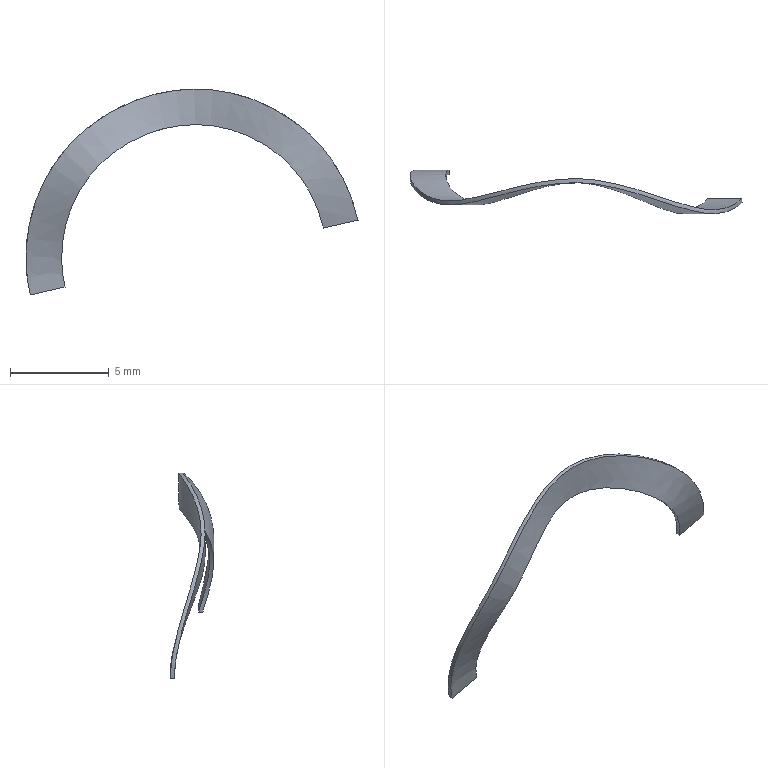Part | NX | features ODD_TURNS_COMBINE 2 | 1 solid | 6 faces | box 16.822 x 2.216 x 10.434 mm | volume 8.771 mm3 | spline 4 | plane 2
STEP:
#1=CARTESIAN_POINT('',(-6.562,-23.97,-1.498));
#2=VERTEX_POINT('',#1);
#3=CARTESIAN_POINT('',(-6.562,-24.173,-1.498));
#4=VERTEX_POINT('',#3);
#5=CARTESIAN_POINT('',(-6.562,-24.173,-1.498));
#6=CARTESIAN_POINT('',(-6.562,-24.105,-1.498));
#7=CARTESIAN_POINT('',(-6.562,-24.037,-1.498));
#8=CARTESIAN_POINT('',(-6.562,-23.97,-1.498));
#9=B_SPLINE_CURVE_WITH_KNOTS('',3,(#5,#6,#7,#8),.UNSPECIFIED.,.F.,.F.,(4,4),(0.000001219,0.0002044),.UNSPECIFIED.);
#10=EDGE_CURVE('',#2,#4,#9,.F.);
#11=ORIENTED_EDGE('',*,*,#10,.T.);
#12=CARTESIAN_POINT('',(-8.32,-24.173,-1.899));
#13=VERTEX_POINT('',#12);
#14=CARTESIAN_POINT('',(-8.32,-24.173,-1.899));
#15=CARTESIAN_POINT('',(-7.734,-24.173,-1.765));
#16=CARTESIAN_POINT('',(-7.148,-24.173,-1.631));
#17=CARTESIAN_POINT('',(-6.562,-24.173,-1.498));
#18=B_SPLINE_CURVE_WITH_KNOTS('',3,(#14,#15,#16,#17),.UNSPECIFIED.,.F.,.F.,(4,4),(0.,0.001803),.UNSPECIFIED.);
#19=EDGE_CURVE('',#4,#13,#18,.F.);
#20=ORIENTED_EDGE('',*,*,#19,.T.);
#21=CARTESIAN_POINT('',(-8.32,-23.97,-1.899));
#22=VERTEX_POINT('',#21);
#23=CARTESIAN_POINT('',(-8.32,-23.97,-1.899));
#24=CARTESIAN_POINT('',(-8.32,-24.037,-1.899));
#25=CARTESIAN_POINT('',(-8.32,-24.105,-1.899));
#26=CARTESIAN_POINT('',(-8.32,-24.173,-1.899));
#27=B_SPLINE_CURVE_WITH_KNOTS('',3,(#23,#24,#25,#26),.UNSPECIFIED.,.F.,.F.,(4,4),(0.,0.0002032),.UNSPECIFIED.);
#28=EDGE_CURVE('',#22,#13,#27,.T.);
#29=ORIENTED_EDGE('',*,*,#28,.F.);
#30=CARTESIAN_POINT('',(-6.562,-23.97,-1.498));
#31=CARTESIAN_POINT('',(-7.148,-23.97,-1.631));
#32=CARTESIAN_POINT('',(-7.734,-23.97,-1.765));
#33=CARTESIAN_POINT('',(-8.32,-23.97,-1.899));
#34=B_SPLINE_CURVE_WITH_KNOTS('',3,(#30,#31,#32,#33),.UNSPECIFIED.,.F.,.F.,(4,4),(0.,0.001803),.UNSPECIFIED.);
#35=EDGE_CURVE('',#22,#2,#34,.F.);
#36=ORIENTED_EDGE('',*,*,#35,.T.);
#37=EDGE_LOOP('',(#11,#20,#29,#36));
#38=FACE_BOUND('',#37,.T.);
#39=CARTESIAN_POINT('',(-8.32,-23.761,-1.899));
#40=DIRECTION('',(0.2225,0.,-0.9749));
#41=DIRECTION('',(-0.9749,0.,-0.2225));
#42=AXIS2_PLACEMENT_3D('',#39,#40,#41);
#43=PLANE('',#42);
#44=ADVANCED_FACE('',(#38),#43,.T.);
#45=CARTESIAN_POINT('',(8.284,-25.419,1.891));
#46=VERTEX_POINT('',#45);
#47=CARTESIAN_POINT('',(-3.703,-25.301,-7.689));
#48=CARTESIAN_POINT('',(-1.417,-25.248,-8.753));
#49=CARTESIAN_POINT('',(4.289,-27.759,-8.773));
#50=CARTESIAN_POINT('',(9.501,-23.516,-2.229));
#51=CARTESIAN_POINT('',(7.592,-27.322,6.131));
#52=CARTESIAN_POINT('',(0.06027,-23.071,9.76));
#53=CARTESIAN_POINT('',(-7.667,-26.878,6.037));
#54=CARTESIAN_POINT('',(-9.528,-22.627,-2.113));
#55=CARTESIAN_POINT('',(-4.18,-26.435,-8.819));
#56=CARTESIAN_POINT('',(4.18,-22.183,-8.819));
#57=CARTESIAN_POINT('',(9.527,-25.991,-2.113));
#58=CARTESIAN_POINT('',(7.668,-21.74,6.038));
#59=CARTESIAN_POINT('',(-0.06063,-25.547,9.759));
#60=CARTESIAN_POINT('',(-7.591,-21.298,6.133));
#61=CARTESIAN_POINT('',(-8.865,-23.825,0.5668));
#62=CARTESIAN_POINT('',(-8.32,-23.761,-1.899));
#63=B_SPLINE_CURVE_WITH_KNOTS('',3,(#47,#48,#49,#50,#51,#52,#53,#54,#55,#56,#57,#58,#59,#60,#61,#62),.UNSPECIFIED.,.F.,.F.,(4,1,1,1,1,1,1,1,1,1,1,1,1,4),(0.,0.07646,0.1539,0.2304,0.3078,0.3843,0.4618,0.5382,0.6157,0.6922,0.7696,0.8461,0.9235,1.),.UNSPECIFIED.);
#64=EDGE_CURVE('',#46,#22,#63,.T.);
#65=ORIENTED_EDGE('',*,*,#64,.T.);
#66=ORIENTED_EDGE('',*,*,#28,.T.);
#67=CARTESIAN_POINT('',(8.284,-25.622,1.891));
#68=VERTEX_POINT('',#67);
#69=CARTESIAN_POINT('',(-3.703,-25.504,-7.689));
#70=CARTESIAN_POINT('',(-1.417,-25.451,-8.753));
#71=CARTESIAN_POINT('',(4.289,-27.962,-8.773));
#72=CARTESIAN_POINT('',(9.501,-23.72,-2.229));
#73=CARTESIAN_POINT('',(7.592,-27.525,6.131));
#74=CARTESIAN_POINT('',(0.06027,-23.274,9.76));
#75=CARTESIAN_POINT('',(-7.667,-27.082,6.037));
#76=CARTESIAN_POINT('',(-9.528,-22.83,-2.113));
#77=CARTESIAN_POINT('',(-4.18,-26.638,-8.819));
#78=CARTESIAN_POINT('',(4.18,-22.387,-8.819));
#79=CARTESIAN_POINT('',(9.527,-26.194,-2.113));
#80=CARTESIAN_POINT('',(7.668,-21.943,6.038));
#81=CARTESIAN_POINT('',(-0.06063,-25.75,9.759));
#82=CARTESIAN_POINT('',(-7.591,-21.501,6.133));
#83=CARTESIAN_POINT('',(-8.865,-24.028,0.5668));
#84=CARTESIAN_POINT('',(-8.32,-23.964,-1.899));
#85=B_SPLINE_CURVE_WITH_KNOTS('',3,(#69,#70,#71,#72,#73,#74,#75,#76,#77,#78,#79,#80,#81,#82,#83,#84),.UNSPECIFIED.,.F.,.F.,(4,1,1,1,1,1,1,1,1,1,1,1,1,4),(0.,0.07646,0.1539,0.2304,0.3078,0.3843,0.4618,0.5382,0.6157,0.6922,0.7696,0.8461,0.9235,1.),.UNSPECIFIED.);
#86=EDGE_CURVE('',#68,#13,#85,.T.);
#87=ORIENTED_EDGE('',*,*,#86,.F.);
#88=CARTESIAN_POINT('',(8.284,-25.622,1.891));
#89=CARTESIAN_POINT('',(8.284,-25.554,1.891));
#90=CARTESIAN_POINT('',(8.284,-25.486,1.891));
#91=CARTESIAN_POINT('',(8.284,-25.419,1.891));
#92=B_SPLINE_CURVE_WITH_KNOTS('',3,(#88,#89,#90,#91),.UNSPECIFIED.,.F.,.F.,(4,4),(0.,0.0002032),.UNSPECIFIED.);
#93=EDGE_CURVE('',#68,#46,#92,.T.);
#94=ORIENTED_EDGE('',*,*,#93,.T.);
#95=EDGE_LOOP('',(#65,#66,#87,#94));
#96=FACE_BOUND('',#95,.T.);
#97=CARTESIAN_POINT('',(8.284,-25.622,1.891));
#98=CARTESIAN_POINT('',(7.999,-25.92,3.139));
#99=CARTESIAN_POINT('',(6.343,-26.82,6.733));
#100=CARTESIAN_POINT('',(0.06027,-23.274,9.76));
#101=CARTESIAN_POINT('',(-7.667,-27.082,6.037));
#102=CARTESIAN_POINT('',(-8.91,-24.241,0.5921));
#103=CARTESIAN_POINT('',(-8.32,-24.173,-1.899));
#104=CARTESIAN_POINT('',(8.284,-25.605,1.891));
#105=CARTESIAN_POINT('',(7.999,-25.903,3.139));
#106=CARTESIAN_POINT('',(6.343,-26.803,6.733));
#107=CARTESIAN_POINT('',(0.06027,-23.257,9.76));
#108=CARTESIAN_POINT('',(-7.667,-27.065,6.037));
#109=CARTESIAN_POINT('',(-8.91,-24.224,0.5921));
#110=CARTESIAN_POINT('',(-8.32,-24.156,-1.899));
#111=CARTESIAN_POINT('',(8.284,-25.571,1.891));
#112=CARTESIAN_POINT('',(7.999,-25.869,3.139));
#113=CARTESIAN_POINT('',(6.343,-26.769,6.733));
#114=CARTESIAN_POINT('',(0.06027,-23.223,9.76));
#115=CARTESIAN_POINT('',(-7.667,-27.031,6.037));
#116=CARTESIAN_POINT('',(-8.91,-24.19,0.5921));
#117=CARTESIAN_POINT('',(-8.32,-24.122,-1.899));
#118=CARTESIAN_POINT('',(8.284,-25.52,1.891));
#119=CARTESIAN_POINT('',(7.999,-25.818,3.139));
#120=CARTESIAN_POINT('',(6.343,-26.718,6.733));
#121=CARTESIAN_POINT('',(0.06027,-23.173,9.76));
#122=CARTESIAN_POINT('',(-7.667,-26.98,6.037));
#123=CARTESIAN_POINT('',(-8.91,-24.14,0.5921));
#124=CARTESIAN_POINT('',(-8.32,-24.071,-1.899));
#125=CARTESIAN_POINT('',(8.284,-25.47,1.891));
#126=CARTESIAN_POINT('',(7.999,-25.767,3.139));
#127=CARTESIAN_POINT('',(6.343,-26.667,6.733));
#128=CARTESIAN_POINT('',(0.06027,-23.122,9.76));
#129=CARTESIAN_POINT('',(-7.667,-26.929,6.037));
#130=CARTESIAN_POINT('',(-8.91,-24.089,0.5921));
#131=CARTESIAN_POINT('',(-8.32,-24.02,-1.899));
#132=CARTESIAN_POINT('',(8.284,-25.436,1.891));
#133=CARTESIAN_POINT('',(7.999,-25.733,3.139));
#134=CARTESIAN_POINT('',(6.343,-26.633,6.733));
#135=CARTESIAN_POINT('',(0.06027,-23.088,9.76));
#136=CARTESIAN_POINT('',(-7.667,-26.895,6.037));
#137=CARTESIAN_POINT('',(-8.91,-24.055,0.5921));
#138=CARTESIAN_POINT('',(-8.32,-23.986,-1.899));
#139=CARTESIAN_POINT('',(8.284,-25.419,1.891));
#140=CARTESIAN_POINT('',(7.999,-25.716,3.139));
#141=CARTESIAN_POINT('',(6.343,-26.616,6.733));
#142=CARTESIAN_POINT('',(0.06027,-23.071,9.76));
#143=CARTESIAN_POINT('',(-7.667,-26.878,6.037));
#144=CARTESIAN_POINT('',(-8.91,-24.038,0.5921));
#145=CARTESIAN_POINT('',(-8.32,-23.97,-1.899));
#146=B_SPLINE_SURFACE_WITH_KNOTS('',3,3,((#97,#98,#99,#100,#101,#102,#103),(#104,#105,#106,#107,#108,#109,#110),(#111,#112,#113,#114,#115,#116,#117),(#118,#119,#120,#121,#122,#123,#124),(#125,#126,#127,#128,#129,#130,#131),(#132,#133,#134,#135,#136,#137,#138),(#139,#140,#141,#142,#143,#144,#145)),.SURF_OF_LINEAR_EXTRUSION.,.F.,.F.,.F.,(4,1,1,1,4),(4,1,1,1,4),(0.,0.25,0.5,0.75,1.),(0.2752,0.3,0.3503,0.4,0.4503),.UNSPECIFIED.);
#147=ADVANCED_FACE('',(#96),#146,.T.);
#148=ORIENTED_EDGE('',*,*,#86,.T.);
#149=ORIENTED_EDGE('',*,*,#19,.F.);
#150=CARTESIAN_POINT('',(6.533,-25.622,1.491));
#151=VERTEX_POINT('',#150);
#152=CARTESIAN_POINT('',(-2.92,-25.504,-6.064));
#153=CARTESIAN_POINT('',(-1.118,-25.451,-6.904));
#154=CARTESIAN_POINT('',(3.383,-27.962,-6.919));
#155=CARTESIAN_POINT('',(7.493,-23.72,-1.758));
#156=CARTESIAN_POINT('',(5.988,-27.525,4.836));
#157=CARTESIAN_POINT('',(0.04752,-23.274,7.697));
#158=CARTESIAN_POINT('',(-6.047,-27.082,4.761));
#159=CARTESIAN_POINT('',(-7.514,-22.83,-1.666));
#160=CARTESIAN_POINT('',(-3.297,-26.638,-6.955));
#161=CARTESIAN_POINT('',(3.297,-22.387,-6.955));
#162=CARTESIAN_POINT('',(7.514,-26.194,-1.666));
#163=CARTESIAN_POINT('',(6.047,-21.943,4.762));
#164=CARTESIAN_POINT('',(-0.04783,-25.75,7.697));
#165=CARTESIAN_POINT('',(-5.987,-21.501,4.837));
#166=CARTESIAN_POINT('',(-6.991,-24.028,0.447));
#167=CARTESIAN_POINT('',(-6.562,-23.964,-1.498));
#168=B_SPLINE_CURVE_WITH_KNOTS('',3,(#152,#153,#154,#155,#156,#157,#158,#159,#160,#161,#162,#163,#164,#165,#166,#167),.UNSPECIFIED.,.F.,.F.,(4,1,1,1,1,1,1,1,1,1,1,1,1,4),(0.,0.07646,0.1539,0.2304,0.3078,0.3843,0.4618,0.5382,0.6157,0.6922,0.7696,0.8461,0.9235,1.),.UNSPECIFIED.);
#169=EDGE_CURVE('',#151,#4,#168,.T.);
#170=ORIENTED_EDGE('',*,*,#169,.F.);
#171=CARTESIAN_POINT('',(6.533,-25.622,1.491));
#172=CARTESIAN_POINT('',(7.117,-25.622,1.624));
#173=CARTESIAN_POINT('',(7.7,-25.622,1.758));
#174=CARTESIAN_POINT('',(8.284,-25.622,1.891));
#175=B_SPLINE_CURVE_WITH_KNOTS('',3,(#171,#172,#173,#174),.UNSPECIFIED.,.F.,.F.,(4,4),(0.,0.001796),.UNSPECIFIED.);
#176=EDGE_CURVE('',#68,#151,#175,.F.);
#177=ORIENTED_EDGE('',*,*,#176,.F.);
#178=EDGE_LOOP('',(#148,#149,#170,#177));
#179=FACE_BOUND('',#178,.T.);
#180=CARTESIAN_POINT('',(6.561,-25.584,1.366));
#181=CARTESIAN_POINT('',(6.345,-25.894,2.396));
#182=CARTESIAN_POINT('',(5.044,-26.849,5.29));
#183=CARTESIAN_POINT('',(0.04752,-23.274,7.697));
#184=CARTESIAN_POINT('',(-6.047,-27.082,4.761));
#185=CARTESIAN_POINT('',(-7.027,-24.241,0.467));
#186=CARTESIAN_POINT('',(-6.562,-24.173,-1.498));
#187=CARTESIAN_POINT('',(6.707,-25.584,1.397));
#188=CARTESIAN_POINT('',(6.487,-25.894,2.449));
#189=CARTESIAN_POINT('',(5.157,-26.849,5.408));
#190=CARTESIAN_POINT('',(0.04858,-23.274,7.869));
#191=CARTESIAN_POINT('',(-6.182,-27.082,4.868));
#192=CARTESIAN_POINT('',(-7.184,-24.241,0.4774));
#193=CARTESIAN_POINT('',(-6.708,-24.173,-1.531));
#194=CARTESIAN_POINT('',(7.,-25.584,1.458));
#195=CARTESIAN_POINT('',(6.77,-25.894,2.556));
#196=CARTESIAN_POINT('',(5.382,-26.849,5.645));
#197=CARTESIAN_POINT('',(0.05071,-23.274,8.213));
#198=CARTESIAN_POINT('',(-6.452,-27.082,5.08));
#199=CARTESIAN_POINT('',(-7.498,-24.241,0.4983));
#200=CARTESIAN_POINT('',(-7.001,-24.173,-1.598));
#201=CARTESIAN_POINT('',(7.44,-25.584,1.549));
#202=CARTESIAN_POINT('',(7.195,-25.894,2.717));
#203=CARTESIAN_POINT('',(5.72,-26.849,5.999));
#204=CARTESIAN_POINT('',(0.05389,-23.274,8.729));
#205=CARTESIAN_POINT('',(-6.857,-27.082,5.399));
#206=CARTESIAN_POINT('',(-7.969,-24.241,0.5296));
#207=CARTESIAN_POINT('',(-7.441,-24.173,-1.698));
#208=CARTESIAN_POINT('',(7.879,-25.584,1.641));
#209=CARTESIAN_POINT('',(7.62,-25.894,2.877));
#210=CARTESIAN_POINT('',(6.058,-26.849,6.353));
#211=CARTESIAN_POINT('',(0.05708,-23.274,9.244));
#212=CARTESIAN_POINT('',(-7.262,-27.082,5.718));
#213=CARTESIAN_POINT('',(-8.439,-24.241,0.5608));
#214=CARTESIAN_POINT('',(-7.88,-24.173,-1.799));
#215=CARTESIAN_POINT('',(8.172,-25.584,1.702));
#216=CARTESIAN_POINT('',(7.903,-25.894,2.984));
#217=CARTESIAN_POINT('',(6.283,-26.849,6.59));
#218=CARTESIAN_POINT('',(0.05921,-23.274,9.588));
#219=CARTESIAN_POINT('',(-7.532,-27.082,5.931));
#220=CARTESIAN_POINT('',(-8.753,-24.241,0.5817));
#221=CARTESIAN_POINT('',(-8.173,-24.173,-1.866));
#222=CARTESIAN_POINT('',(8.319,-25.584,1.732));
#223=CARTESIAN_POINT('',(8.045,-25.894,3.038));
#224=CARTESIAN_POINT('',(6.396,-26.849,6.708));
#225=CARTESIAN_POINT('',(0.06027,-23.274,9.76));
#226=CARTESIAN_POINT('',(-7.667,-27.082,6.037));
#227=CARTESIAN_POINT('',(-8.91,-24.241,0.5921));
#228=CARTESIAN_POINT('',(-8.32,-24.173,-1.899));
#229=B_SPLINE_SURFACE_WITH_KNOTS('',3,3,((#180,#181,#182,#183,#184,#185,#186),(#187,#188,#189,#190,#191,#192,#193),(#194,#195,#196,#197,#198,#199,#200),(#201,#202,#203,#204,#205,#206,#207),(#208,#209,#210,#211,#212,#213,#214),(#215,#216,#217,#218,#219,#220,#221),(#222,#223,#224,#225,#226,#227,#228)),.RULED_SURF.,.F.,.F.,.F.,(4,1,1,1,4),(4,1,1,1,4),(0.,0.25,0.5,0.75,1.),(0.2741,0.3,0.3503,0.4,0.4503),.UNSPECIFIED.);
#230=ADVANCED_FACE('',(#179),#229,.T.);
#231=CARTESIAN_POINT('',(6.533,-25.419,1.491));
#232=VERTEX_POINT('',#231);
#233=CARTESIAN_POINT('',(-2.92,-25.301,-6.064));
#234=CARTESIAN_POINT('',(-1.118,-25.248,-6.904));
#235=CARTESIAN_POINT('',(3.383,-27.759,-6.919));
#236=CARTESIAN_POINT('',(7.493,-23.516,-1.758));
#237=CARTESIAN_POINT('',(5.988,-27.322,4.836));
#238=CARTESIAN_POINT('',(0.04752,-23.071,7.697));
#239=CARTESIAN_POINT('',(-6.047,-26.878,4.761));
#240=CARTESIAN_POINT('',(-7.514,-22.627,-1.666));
#241=CARTESIAN_POINT('',(-3.297,-26.435,-6.955));
#242=CARTESIAN_POINT('',(3.297,-22.183,-6.955));
#243=CARTESIAN_POINT('',(7.514,-25.991,-1.666));
#244=CARTESIAN_POINT('',(6.047,-21.74,4.762));
#245=CARTESIAN_POINT('',(-0.04783,-25.547,7.697));
#246=CARTESIAN_POINT('',(-5.987,-21.298,4.837));
#247=CARTESIAN_POINT('',(-6.991,-23.825,0.447));
#248=CARTESIAN_POINT('',(-6.562,-23.761,-1.498));
#249=B_SPLINE_CURVE_WITH_KNOTS('',3,(#233,#234,#235,#236,#237,#238,#239,#240,#241,#242,#243,#244,#245,#246,#247,#248),.UNSPECIFIED.,.F.,.F.,(4,1,1,1,1,1,1,1,1,1,1,1,1,4),(0.,0.07646,0.1539,0.2304,0.3078,0.3843,0.4618,0.5382,0.6157,0.6922,0.7696,0.8461,0.9235,1.),.UNSPECIFIED.);
#250=EDGE_CURVE('',#232,#2,#249,.T.);
#251=ORIENTED_EDGE('',*,*,#250,.T.);
#252=ORIENTED_EDGE('',*,*,#35,.F.);
#253=ORIENTED_EDGE('',*,*,#64,.F.);
#254=CARTESIAN_POINT('',(8.284,-25.419,1.891));
#255=CARTESIAN_POINT('',(7.7,-25.419,1.758));
#256=CARTESIAN_POINT('',(7.117,-25.419,1.624));
#257=CARTESIAN_POINT('',(6.533,-25.419,1.491));
#258=B_SPLINE_CURVE_WITH_KNOTS('',3,(#254,#255,#256,#257),.UNSPECIFIED.,.F.,.F.,(4,4),(0.,0.001796),.UNSPECIFIED.);
#259=EDGE_CURVE('',#232,#46,#258,.F.);
#260=ORIENTED_EDGE('',*,*,#259,.F.);
#261=EDGE_LOOP('',(#251,#252,#253,#260));
#262=FACE_BOUND('',#261,.T.);
#263=CARTESIAN_POINT('',(8.319,-25.381,1.732));
#264=CARTESIAN_POINT('',(8.045,-25.691,3.038));
#265=CARTESIAN_POINT('',(6.396,-26.646,6.708));
#266=CARTESIAN_POINT('',(0.06027,-23.071,9.76));
#267=CARTESIAN_POINT('',(-7.667,-26.878,6.037));
#268=CARTESIAN_POINT('',(-8.91,-24.038,0.5921));
#269=CARTESIAN_POINT('',(-8.32,-23.97,-1.899));
#270=CARTESIAN_POINT('',(8.246,-25.381,1.717));
#271=CARTESIAN_POINT('',(7.974,-25.691,3.011));
#272=CARTESIAN_POINT('',(6.339,-26.646,6.649));
#273=CARTESIAN_POINT('',(0.05974,-23.071,9.674));
#274=CARTESIAN_POINT('',(-7.6,-26.878,5.984));
#275=CARTESIAN_POINT('',(-8.832,-24.038,0.5869));
#276=CARTESIAN_POINT('',(-8.247,-23.97,-1.882));
#277=CARTESIAN_POINT('',(8.099,-25.381,1.686));
#278=CARTESIAN_POINT('',(7.833,-25.691,2.958));
#279=CARTESIAN_POINT('',(6.227,-26.646,6.531));
#280=CARTESIAN_POINT('',(0.05867,-23.071,9.502));
#281=CARTESIAN_POINT('',(-7.465,-26.878,5.878));
#282=CARTESIAN_POINT('',(-8.675,-24.038,0.5765));
#283=CARTESIAN_POINT('',(-8.1,-23.97,-1.849));
#284=CARTESIAN_POINT('',(7.879,-25.381,1.641));
#285=CARTESIAN_POINT('',(7.62,-25.691,2.877));
#286=CARTESIAN_POINT('',(6.058,-26.646,6.353));
#287=CARTESIAN_POINT('',(0.05708,-23.071,9.244));
#288=CARTESIAN_POINT('',(-7.262,-26.878,5.718));
#289=CARTESIAN_POINT('',(-8.439,-24.038,0.5608));
#290=CARTESIAN_POINT('',(-7.88,-23.97,-1.799));
#291=CARTESIAN_POINT('',(7.66,-25.381,1.595));
#292=CARTESIAN_POINT('',(7.408,-25.691,2.797));
#293=CARTESIAN_POINT('',(5.889,-26.646,6.176));
#294=CARTESIAN_POINT('',(0.05549,-23.071,8.986));
#295=CARTESIAN_POINT('',(-7.06,-26.878,5.559));
#296=CARTESIAN_POINT('',(-8.204,-24.038,0.5452));
#297=CARTESIAN_POINT('',(-7.661,-23.97,-1.748));
#298=CARTESIAN_POINT('',(7.513,-25.381,1.564));
#299=CARTESIAN_POINT('',(7.266,-25.691,2.744));
#300=CARTESIAN_POINT('',(5.776,-26.646,6.058));
#301=CARTESIAN_POINT('',(0.05442,-23.071,8.815));
#302=CARTESIAN_POINT('',(-6.925,-26.878,5.453));
#303=CARTESIAN_POINT('',(-8.047,-24.038,0.5348));
#304=CARTESIAN_POINT('',(-7.514,-23.97,-1.715));
#305=CARTESIAN_POINT('',(7.367,-25.381,1.534));
#306=CARTESIAN_POINT('',(7.124,-25.691,2.69));
#307=CARTESIAN_POINT('',(5.664,-26.646,5.94));
#308=CARTESIAN_POINT('',(0.05336,-23.071,8.643));
#309=CARTESIAN_POINT('',(-6.79,-26.878,5.346));
#310=CARTESIAN_POINT('',(-7.89,-24.038,0.5243));
#311=CARTESIAN_POINT('',(-7.368,-23.97,-1.682));
#312=CARTESIAN_POINT('',(7.22,-25.381,1.503));
#313=CARTESIAN_POINT('',(6.983,-25.691,2.637));
#314=CARTESIAN_POINT('',(5.551,-26.646,5.822));
#315=CARTESIAN_POINT('',(0.0523,-23.071,8.471));
#316=CARTESIAN_POINT('',(-6.655,-26.878,5.24));
#317=CARTESIAN_POINT('',(-7.733,-24.038,0.5139));
#318=CARTESIAN_POINT('',(-7.221,-23.97,-1.648));
#319=CARTESIAN_POINT('',(7.,-25.381,1.458));
#320=CARTESIAN_POINT('',(6.77,-25.691,2.556));
#321=CARTESIAN_POINT('',(5.382,-26.646,5.645));
#322=CARTESIAN_POINT('',(0.05071,-23.071,8.213));
#323=CARTESIAN_POINT('',(-6.452,-26.878,5.08));
#324=CARTESIAN_POINT('',(-7.498,-24.038,0.4983));
#325=CARTESIAN_POINT('',(-7.001,-23.97,-1.598));
#326=CARTESIAN_POINT('',(6.781,-25.381,1.412));
#327=CARTESIAN_POINT('',(6.558,-25.691,2.476));
#328=CARTESIAN_POINT('',(5.213,-26.646,5.468));
#329=CARTESIAN_POINT('',(0.04911,-23.071,7.955));
#330=CARTESIAN_POINT('',(-6.25,-26.878,4.921));
#331=CARTESIAN_POINT('',(-7.263,-24.038,0.4826));
#332=CARTESIAN_POINT('',(-6.782,-23.97,-1.548));
#333=CARTESIAN_POINT('',(6.634,-25.381,1.381));
#334=CARTESIAN_POINT('',(6.416,-25.691,2.423));
#335=CARTESIAN_POINT('',(5.1,-26.646,5.349));
#336=CARTESIAN_POINT('',(0.04805,-23.071,7.783));
#337=CARTESIAN_POINT('',(-6.115,-26.878,4.815));
#338=CARTESIAN_POINT('',(-7.106,-24.038,0.4722));
#339=CARTESIAN_POINT('',(-6.635,-23.97,-1.514));
#340=CARTESIAN_POINT('',(6.561,-25.381,1.366));
#341=CARTESIAN_POINT('',(6.345,-25.691,2.396));
#342=CARTESIAN_POINT('',(5.044,-26.646,5.29));
#343=CARTESIAN_POINT('',(0.04752,-23.071,7.697));
#344=CARTESIAN_POINT('',(-6.047,-26.878,4.761));
#345=CARTESIAN_POINT('',(-7.027,-24.038,0.467));
#346=CARTESIAN_POINT('',(-6.562,-23.97,-1.498));
#347=B_SPLINE_SURFACE_WITH_KNOTS('',3,3,((#263,#264,#265,#266,#267,#268,#269),(#270,#271,#272,#273,#274,#275,#276),(#277,#278,#279,#280,#281,#282,#283),(#284,#285,#286,#287,#288,#289,#290),(#291,#292,#293,#294,#295,#296,#297),(#298,#299,#300,#301,#302,#303,#304),(#305,#306,#307,#308,#309,#310,#311),(#312,#313,#314,#315,#316,#317,#318),(#319,#320,#321,#322,#323,#324,#325),(#326,#327,#328,#329,#330,#331,#332),(#333,#334,#335,#336,#337,#338,#339),(#340,#341,#342,#343,#344,#345,#346)),.RULED_SURF.,.F.,.F.,.F.,(4,1,1,1,2,1,1,1,4),(4,1,1,1,4),(0.,0.125,0.25,0.375,0.5,0.625,0.75,0.875,1.),(0.2741,0.3,0.3503,0.4,0.4503),.UNSPECIFIED.);
#348=ADVANCED_FACE('',(#262),#347,.T.);
#349=ORIENTED_EDGE('',*,*,#169,.T.);
#350=ORIENTED_EDGE('',*,*,#10,.F.);
#351=ORIENTED_EDGE('',*,*,#250,.F.);
#352=CARTESIAN_POINT('',(6.533,-25.419,1.491));
#353=CARTESIAN_POINT('',(6.533,-25.486,1.491));
#354=CARTESIAN_POINT('',(6.533,-25.554,1.491));
#355=CARTESIAN_POINT('',(6.533,-25.622,1.491));
#356=B_SPLINE_CURVE_WITH_KNOTS('',3,(#352,#353,#354,#355),.UNSPECIFIED.,.F.,.F.,(4,4),(0.,0.0002032),.UNSPECIFIED.);
#357=EDGE_CURVE('',#151,#232,#356,.F.);
#358=ORIENTED_EDGE('',*,*,#357,.F.);
#359=EDGE_LOOP('',(#349,#350,#351,#358));
#360=FACE_BOUND('',#359,.T.);
#361=CARTESIAN_POINT('',(6.533,-25.419,1.491));
#362=CARTESIAN_POINT('',(6.309,-25.716,2.475));
#363=CARTESIAN_POINT('',(5.002,-26.616,5.31));
#364=CARTESIAN_POINT('',(0.04752,-23.071,7.697));
#365=CARTESIAN_POINT('',(-6.047,-26.878,4.761));
#366=CARTESIAN_POINT('',(-7.027,-24.038,0.467));
#367=CARTESIAN_POINT('',(-6.562,-23.97,-1.498));
#368=CARTESIAN_POINT('',(6.533,-25.436,1.491));
#369=CARTESIAN_POINT('',(6.309,-25.733,2.475));
#370=CARTESIAN_POINT('',(5.002,-26.633,5.31));
#371=CARTESIAN_POINT('',(0.04752,-23.088,7.697));
#372=CARTESIAN_POINT('',(-6.047,-26.895,4.761));
#373=CARTESIAN_POINT('',(-7.027,-24.055,0.467));
#374=CARTESIAN_POINT('',(-6.562,-23.986,-1.498));
#375=CARTESIAN_POINT('',(6.533,-25.47,1.491));
#376=CARTESIAN_POINT('',(6.309,-25.767,2.475));
#377=CARTESIAN_POINT('',(5.002,-26.667,5.31));
#378=CARTESIAN_POINT('',(0.04752,-23.122,7.697));
#379=CARTESIAN_POINT('',(-6.047,-26.929,4.761));
#380=CARTESIAN_POINT('',(-7.027,-24.089,0.467));
#381=CARTESIAN_POINT('',(-6.562,-24.02,-1.498));
#382=CARTESIAN_POINT('',(6.533,-25.52,1.491));
#383=CARTESIAN_POINT('',(6.309,-25.818,2.475));
#384=CARTESIAN_POINT('',(5.002,-26.718,5.31));
#385=CARTESIAN_POINT('',(0.04752,-23.173,7.697));
#386=CARTESIAN_POINT('',(-6.047,-26.98,4.761));
#387=CARTESIAN_POINT('',(-7.027,-24.14,0.467));
#388=CARTESIAN_POINT('',(-6.562,-24.071,-1.498));
#389=CARTESIAN_POINT('',(6.533,-25.571,1.491));
#390=CARTESIAN_POINT('',(6.309,-25.869,2.475));
#391=CARTESIAN_POINT('',(5.002,-26.769,5.31));
#392=CARTESIAN_POINT('',(0.04752,-23.223,7.697));
#393=CARTESIAN_POINT('',(-6.047,-27.031,4.761));
#394=CARTESIAN_POINT('',(-7.027,-24.19,0.467));
#395=CARTESIAN_POINT('',(-6.562,-24.122,-1.498));
#396=CARTESIAN_POINT('',(6.533,-25.605,1.491));
#397=CARTESIAN_POINT('',(6.309,-25.903,2.475));
#398=CARTESIAN_POINT('',(5.002,-26.803,5.31));
#399=CARTESIAN_POINT('',(0.04752,-23.257,7.697));
#400=CARTESIAN_POINT('',(-6.047,-27.065,4.761));
#401=CARTESIAN_POINT('',(-7.027,-24.224,0.467));
#402=CARTESIAN_POINT('',(-6.562,-24.156,-1.498));
#403=CARTESIAN_POINT('',(6.533,-25.622,1.491));
#404=CARTESIAN_POINT('',(6.309,-25.92,2.475));
#405=CARTESIAN_POINT('',(5.002,-26.82,5.31));
#406=CARTESIAN_POINT('',(0.04752,-23.274,7.697));
#407=CARTESIAN_POINT('',(-6.047,-27.082,4.761));
#408=CARTESIAN_POINT('',(-7.027,-24.241,0.467));
#409=CARTESIAN_POINT('',(-6.562,-24.173,-1.498));
#410=B_SPLINE_SURFACE_WITH_KNOTS('',3,3,((#361,#362,#363,#364,#365,#366,#367),(#368,#369,#370,#371,#372,#373,#374),(#375,#376,#377,#378,#379,#380,#381),(#382,#383,#384,#385,#386,#387,#388),(#389,#390,#391,#392,#393,#394,#395),(#396,#397,#398,#399,#400,#401,#402),(#403,#404,#405,#406,#407,#408,#409)),.SURF_OF_LINEAR_EXTRUSION.,.F.,.F.,.F.,(4,1,1,1,4),(4,1,1,1,4),(0.,0.25,0.5,0.75,1.),(0.2752,0.3,0.3503,0.4,0.4503),.UNSPECIFIED.);
#411=ADVANCED_FACE('',(#360),#410,.T.);
#412=ORIENTED_EDGE('',*,*,#357,.T.);
#413=ORIENTED_EDGE('',*,*,#259,.T.);
#414=ORIENTED_EDGE('',*,*,#93,.F.);
#415=ORIENTED_EDGE('',*,*,#176,.T.);
#416=EDGE_LOOP('',(#412,#413,#414,#415));
#417=FACE_BOUND('',#416,.T.);
#418=CARTESIAN_POINT('',(-8.32,-23.761,-1.899));
#419=DIRECTION('',(0.2225,0.,-0.9749));
#420=DIRECTION('',(-0.9749,0.,-0.2225));
#421=AXIS2_PLACEMENT_3D('',#418,#419,#420);
#422=PLANE('',#421);
#423=ADVANCED_FACE('',(#417),#422,.T.);
#424=CLOSED_SHELL('',(#44,#147,#230,#348,#411,#423));
#425=MANIFOLD_SOLID_BREP('',#424);
#426=(LENGTH_UNIT()NAMED_UNIT(*)SI_UNIT(.MILLI.,.METRE.));
#427=UNCERTAINTY_MEASURE_WITH_UNIT(LENGTH_MEASURE(0.0508),#426,'','');
#428=(NAMED_UNIT(*)PLANE_ANGLE_UNIT()SI_UNIT($,.RADIAN.));
#429=(NAMED_UNIT(*)SI_UNIT($,.STERADIAN.)SOLID_ANGLE_UNIT());
#430=(GEOMETRIC_REPRESENTATION_CONTEXT(3)GLOBAL_UNCERTAINTY_ASSIGNED_CONTEXT((#427))GLOBAL_UNIT_ASSIGNED_CONTEXT((#426,#428,#429))REPRESENTATION_CONTEXT('',''));
#431=ADVANCED_BREP_SHAPE_REPRESENTATION('',(#425),#430);